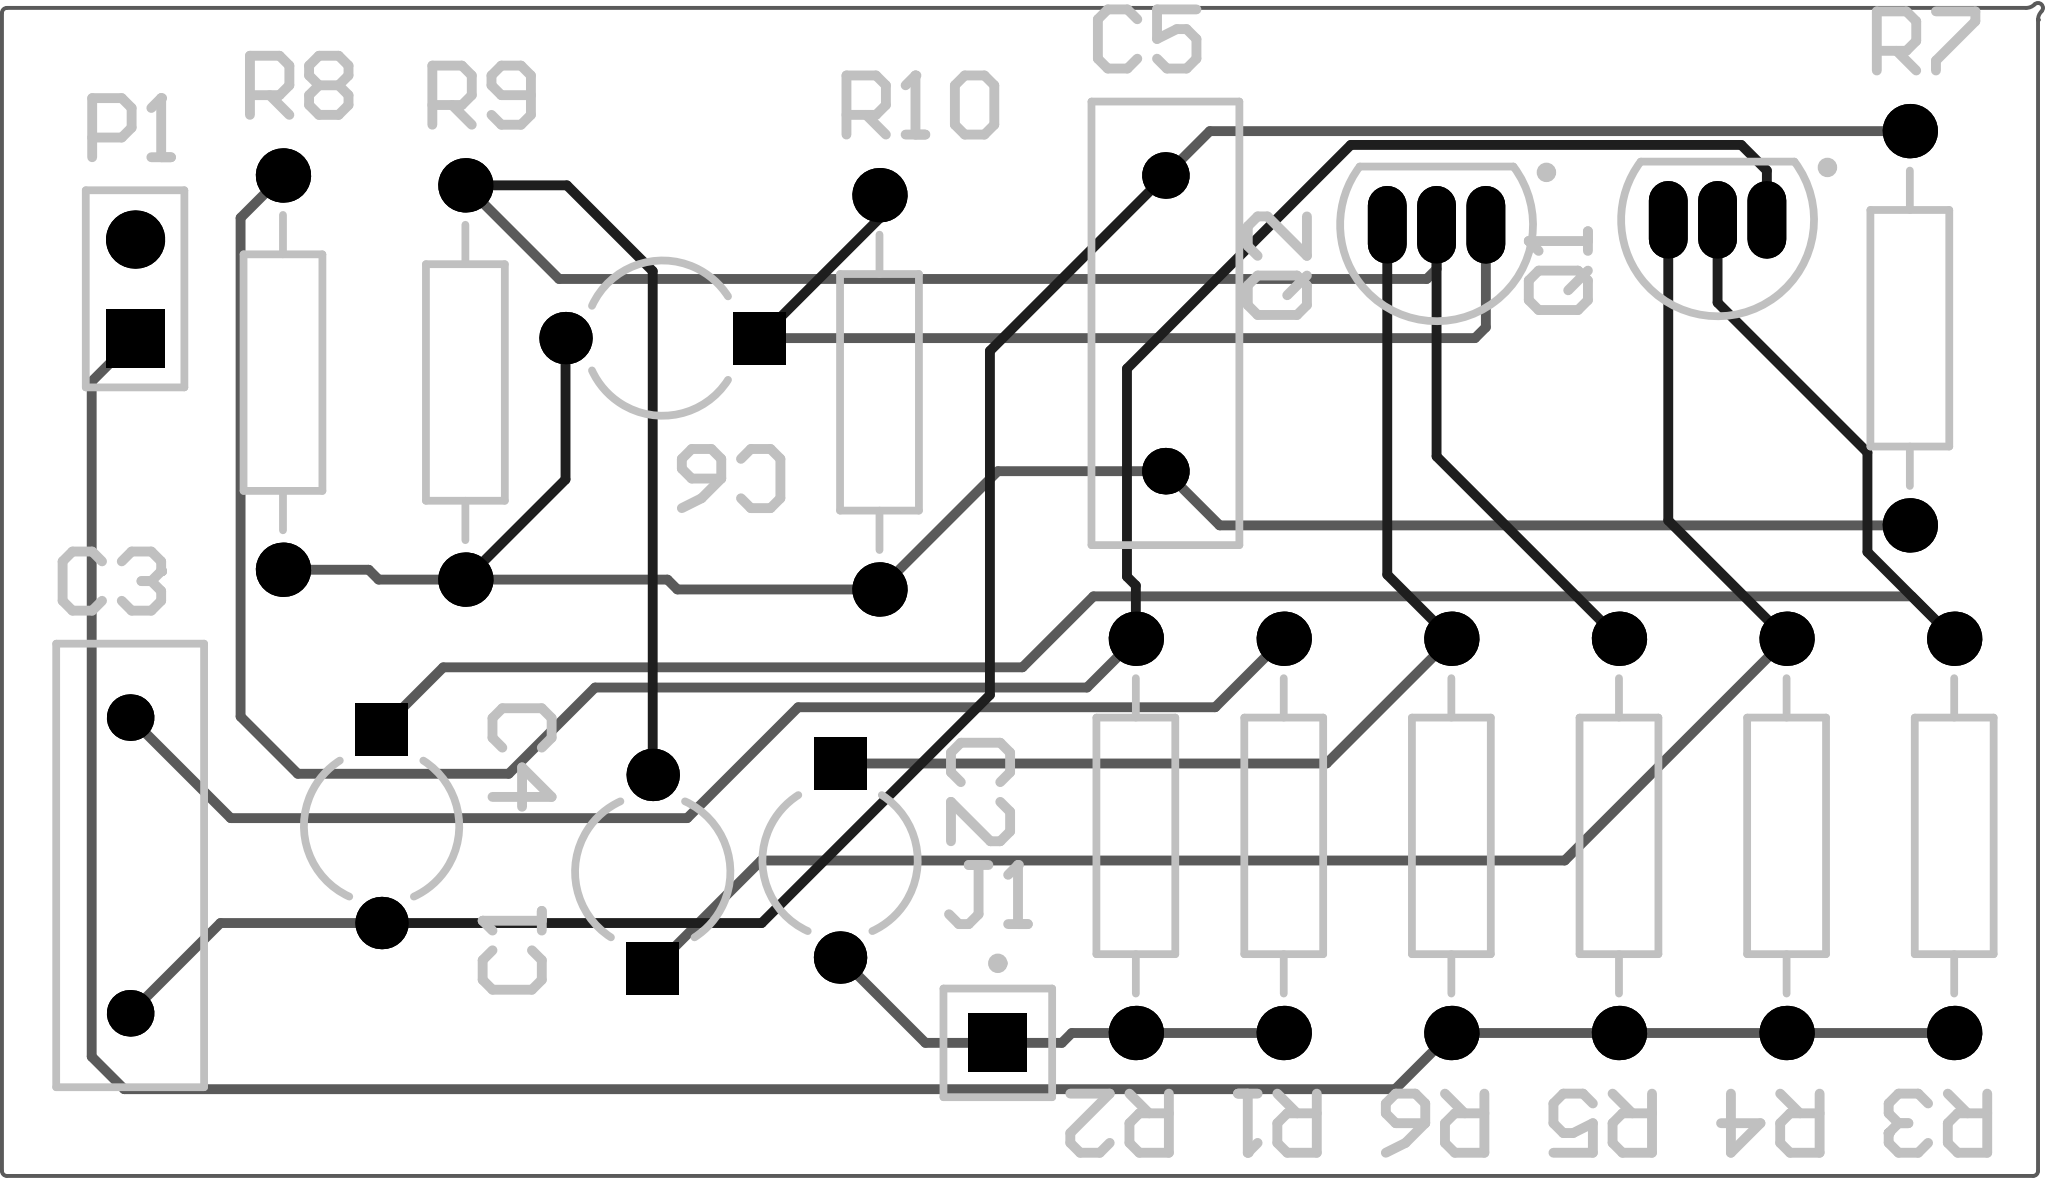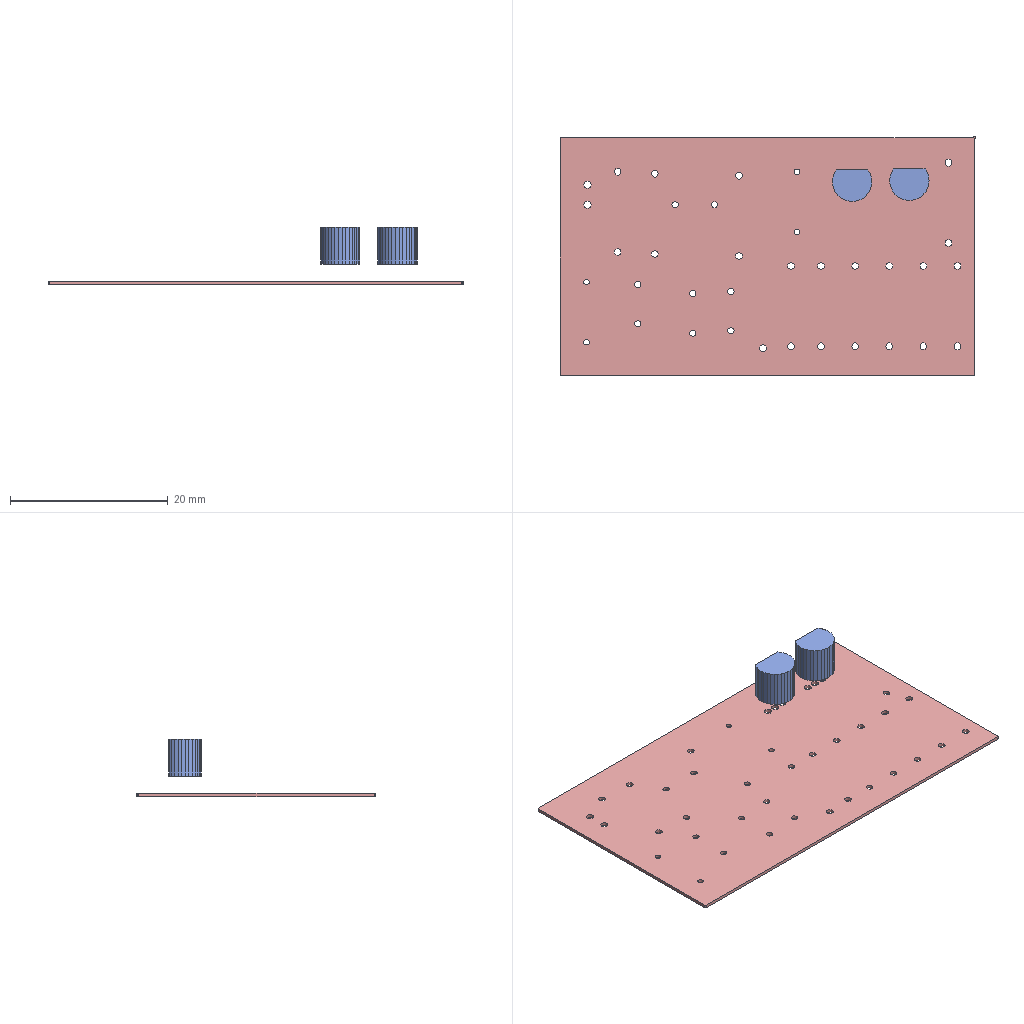Circuit board layout | Altium Designer | box 52.6 x 30.2 x 7.3 mm
Layer stack:
# Altium Designer layer stack of  (unit mm; dielectric type: 0 none, 1 core, 2 prepreg, 3 surface material)
index,name,kind,layer,copper_thickness_mm,dielectric_type,dielectric_thickness_mm,dielectric_material,dielectric_constant
0,Top Paste,other,,,,,,
1,Top Overlay,other,,,,,,
2,Top Solder,dielectric,,,3,0.0102,Solder Resist,3.5
3,Top Layer,copper,Top Layer,0.0356,,,,
4,Dielectric 1,dielectric,,,0,0.32,FR-4,4.8
5,Bottom Layer,copper,Bottom Layer,0.0356,,,,
6,Bottom Solder,dielectric,,,3,0.0102,Solder Resist,3.5
7,Bottom Overlay,other,,,,,,
8,Bottom Paste,other,,,,,,
# drill layer pairs: low layer,high layer
drill_pair,Top Layer,Bottom Layer
Part placement:
Designator,Comment,Layer,Footprint,Center-X(mm),Center-Y(mm),Rotation
R10,470,TopLayer,AXIAL-0.4,64.77,74.041,90
R9,10K,TopLayer,AXIAL-0.4,54.102,74.295,90
R8,1.2K,TopLayer,AXIAL-0.4,49.403,74.549,90
R7,16K,TopLayer,AXIAL-0.4,91.313,75.692,90
R6,5.1K,TopLayer,AXIAL-0.4,79.502,62.611,270
R5,10K,TopLayer,AXIAL-0.4,83.82,62.611,270
R4,10K,TopLayer,AXIAL-0.4,88.138,62.611,270
R3,10K,TopLayer,AXIAL-0.4,92.456,62.611,270
R2,10K,TopLayer,AXIAL-0.4,71.374,62.611,270
R1,16K,TopLayer,AXIAL-0.4,75.184,62.611,270
Q2,9013,TopLayer,TO-92A,79.121,78.359,90
Q1,9013,TopLayer,TO-92A,86.36,78.486,90
P1,Header 2,TopLayer,HDR1X2,45.593,76.708,90
J1,Socket,TopLayer,PIN1,67.818,57.277,0
C6,10uF,TopLayer,CAPR5-4X5,59.182,75.438,180
C5,0.01uF,TopLayer,RAD-0.3,72.136,75.819,90
C4,10uF,TopLayer,CAPR5-4X5,51.943,62.865,270
C3,0.01uF,TopLayer,RAD-0.3,45.466,61.849,90
C2,10uF,TopLayer,CAPR5-4X5,63.754,61.976,270
C1,10uF,TopLayer,CAPR5-4X5,58.928,61.682,90
Pad and via stacks:
# Altium Designer via and pad stacks of  (unit mm). Each distinct definition once, with the count of objects using it.
# via: kind,start_layer,end_layer,hole_mm,diameter_mm,mode(0 simple;1 top-mid-bottom;2 full stack),diameter_per_layer,count,example_net
# pad: kind,layer,hole_mm,hole_type(0 round;1 square;2 slot),plating,top_size,top_shape(1 round;2 rect;3 octagon;9 rounded rect),mid_size,bottom_size,mode,footprint,size_per_layer,count,example
pad,Multi-Layer,0.85,0,plated,1.4x1.4,1,1.4x1.4,1.4x1.4,0,AXIAL-0.4,,20,R2.1
pad,Multi-Layer,0.9,0,plated,1.5x1.5,2,1.5x1.5,1.5x1.5,0,PIN1,,1,J1.1
pad,Multi-Layer,0.8,0,plated,1.35x1.35,1,1.35x1.35,1.35x1.35,0,CAPR5-4X5,,4,C2.2
pad,Multi-Layer,0.8,0,plated,1.35x1.35,2,1.35x1.35,1.35x1.35,0,CAPR5-4X5,,4,C2.1
pad,Multi-Layer,0.7,0,plated,1.2x1.2,1,1.2x1.2,1.2x1.2,0,RAD-0.3,,4,C3.2
pad,Multi-Layer,0.9,0,plated,2x1,1,2x1,2x1,0,TO-92A,,6,Q2.3
pad,Multi-Layer,0.9,0,plated,1.5x1.5,2,1.5x1.5,1.5x1.5,0,HDR1X2,,1,P1.1
pad,Multi-Layer,0.9,0,plated,1.5x1.5,1,1.5x1.5,1.5x1.5,0,HDR1X2,,1,P1.2
Design rules, without the lines most boards share:
# Altium Designer design rules of  (exported by Altium Designer, unit mm)
# columns: name | kind | enabled | priority | scope1 | scope2 | descriptor | typed fields (field=value)
HoleToHoleClearance | 52 | enabled | 1 | All | All | Hole To Hole Clearance (Gap=10mil) (All),(All) | gap=0.254
DiffPairsRouting | 51 | enabled | 1 | All | All | Differential Pairs Uncoupled Length using the Gap Constraints (Min=10mil) (Max=10mil) (Prefered=10mil)  and Width Constraints (Min=15mil) (Max=15mil) (Prefered=15mil) (All) |
SolderMaskExpansion | 13 | enabled | 1 | All | All | Solder Mask Expansion (Expansion =4mil) (All) | expansion=0.1016
PasteMaskExpansion | 14 | enabled | 1 | All | All | Paste Mask Expansion (Expansion =0mil) (All) | expansion=0
RoutingVias | 11 | enabled | 1 | All | All | Routing Via (MinHoleWidth=28mil) (MaxHoleWidth=28mil) (PreferredHoleWidth=28mil) (MinWidth=50mil) (MaxWidth=50mil) (PreferedWidth=50mil) (All) | via_min_hole=0.7112 via_max_hole=0.7112 via_preferred_diameter=1.27 via_preferred_hole=0.7112
Width | 2 | enabled | 1 | All | All | Width Constraint (Min=10mil) (Max=10mil) (Preferred=10mil) (All) |
PolygonConnect | 20 | enabled | 1 | All | All | Polygon Connect Rule(Relief Connect )(Conductor Width=10mil) (Relief Angle=90 Angle) (Entries=4) (Air Gap Width=10mil) (All),(All) | connect_style(0=relief,1=direct,2=none)=0 relief_conductor_width=0.254 relief_entries=4
PlaneConnect | 6 | enabled | 1 | All | All | Power Plane Connect Rule(Relief Connect )(Expansion=20mil) (Conductor Width=10mil) (Air Gap=10mil) (Entries=4) (All) | relief_conductor_width=0.254 relief_entries=4 relief_expansion=0.508
Clearance | 0 | enabled | 1 | All | All | Clearance Constraint (Gap=10mil) (All),(All) | gap=0.254
Classes set for this board:
# Altium Designer classes of  (member kind: 0 net, 1 component, 2 from-to, 3 pad, 4 layer, 5 differential pair, 6 design channel, 7 polygon, 8 structure, 9 xSignal)
# columns: class name | member kind | superclass | members
Sheet2 | 1 | no | C1; C2; C3; C4; C5; C6; J1; P1; Q1; Q2; R1; R2; R3; R4; R5; R6; R7; R8; R9; R10;